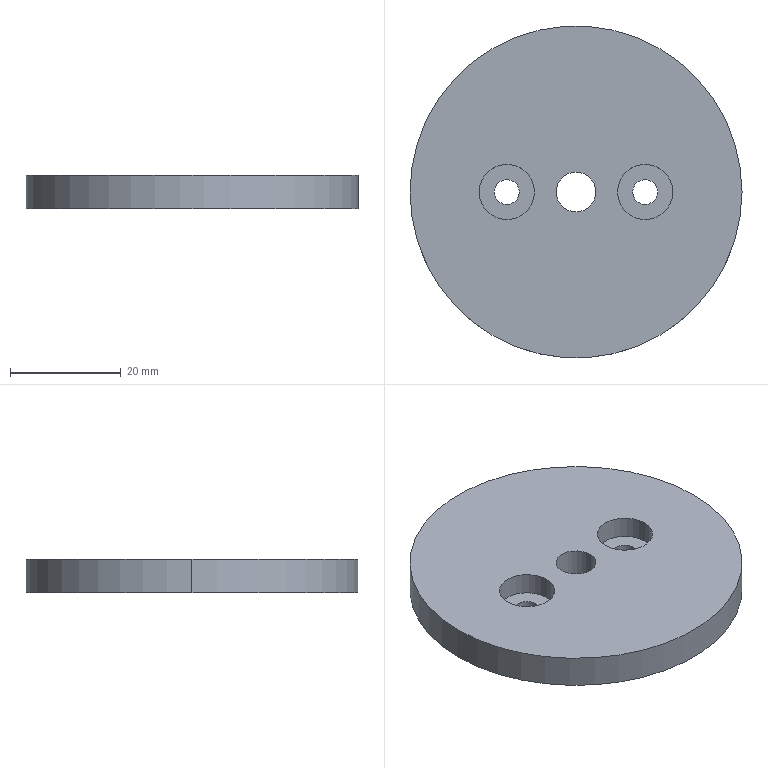Part | SolidWorks | features Extrusion 1, HoleWzd 1, ICE 1 | 1 solid | 16 faces | box 60 x 60 x 6 mm | volume 16028 mm3 | cylinder 12 | plane 4 | commonest cylinder face diameters 4.5 x4 10 x4 7.2 x2 60 x2
STEP:
#1=CARTESIAN_POINT('',(-3.6,0.,0.));
#2=VERTEX_POINT('',#1);
#3=CARTESIAN_POINT('',(3.6,0.,0.));
#4=VERTEX_POINT('',#3);
#5=CARTESIAN_POINT('',(0.,0.,0.));
#6=DIRECTION('',(0.,0.,1.));
#7=DIRECTION('',(1.,0.,0.));
#8=AXIS2_PLACEMENT_3D('',#5,#6,#7);
#9=CIRCLE('',#8,3.6);
#10=EDGE_CURVE('',#2,#4,#9,.T.);
#11=ORIENTED_EDGE('',*,*,#10,.F.);
#12=CARTESIAN_POINT('',(-3.6,0.,6.));
#13=VERTEX_POINT('',#12);
#14=CARTESIAN_POINT('',(-3.6,0.,-4.));
#15=DIRECTION('',(0.,0.,1.));
#16=VECTOR('',#15,1000.);
#17=LINE('',#14,#16);
#18=EDGE_CURVE('',#2,#13,#17,.T.);
#19=ORIENTED_EDGE('',*,*,#18,.T.);
#20=CARTESIAN_POINT('',(3.6,0.,6.));
#21=VERTEX_POINT('',#20);
#22=CARTESIAN_POINT('',(0.,0.,6.));
#23=DIRECTION('',(0.,0.,1.));
#24=DIRECTION('',(1.,0.,0.));
#25=AXIS2_PLACEMENT_3D('',#22,#23,#24);
#26=CIRCLE('',#25,3.6);
#27=EDGE_CURVE('',#13,#21,#26,.T.);
#28=ORIENTED_EDGE('',*,*,#27,.T.);
#29=CARTESIAN_POINT('',(3.6,0.,-4.));
#30=DIRECTION('',(0.,0.,1.));
#31=VECTOR('',#30,1000.);
#32=LINE('',#29,#31);
#33=EDGE_CURVE('',#4,#21,#32,.T.);
#34=ORIENTED_EDGE('',*,*,#33,.F.);
#35=EDGE_LOOP('',(#11,#19,#28,#34));
#36=FACE_OUTER_BOUND('',#35,.T.);
#37=CARTESIAN_POINT('',(0.,0.,-4.));
#38=DIRECTION('',(0.,0.,1.));
#39=DIRECTION('',(1.,0.,0.));
#40=AXIS2_PLACEMENT_3D('',#37,#38,#39);
#41=CYLINDRICAL_SURFACE('',#40,3.6);
#42=ADVANCED_FACE('',(#36),#41,.F.);
#43=CARTESIAN_POINT('',(-17.5,0.,2.));
#44=VERTEX_POINT('',#43);
#45=CARTESIAN_POINT('',(-7.5,0.,2.));
#46=VERTEX_POINT('',#45);
#47=CARTESIAN_POINT('',(-12.5,0.,2.));
#48=DIRECTION('',(0.,0.,1.));
#49=DIRECTION('',(1.,0.,0.));
#50=AXIS2_PLACEMENT_3D('',#47,#48,#49);
#51=CIRCLE('',#50,5.);
#52=EDGE_CURVE('',#44,#46,#51,.T.);
#53=ORIENTED_EDGE('',*,*,#52,.F.);
#54=CARTESIAN_POINT('',(-17.5,0.,6.));
#55=VERTEX_POINT('',#54);
#56=CARTESIAN_POINT('',(-17.5,0.,6.));
#57=DIRECTION('',(0.,0.,1.));
#58=VECTOR('',#57,1000.);
#59=LINE('',#56,#58);
#60=EDGE_CURVE('',#44,#55,#59,.T.);
#61=ORIENTED_EDGE('',*,*,#60,.T.);
#62=CARTESIAN_POINT('',(-7.5,0.,6.));
#63=VERTEX_POINT('',#62);
#64=CARTESIAN_POINT('',(-12.5,0.,6.));
#65=DIRECTION('',(0.,0.,1.));
#66=DIRECTION('',(1.,0.,0.));
#67=AXIS2_PLACEMENT_3D('',#64,#65,#66);
#68=CIRCLE('',#67,5.);
#69=EDGE_CURVE('',#55,#63,#68,.T.);
#70=ORIENTED_EDGE('',*,*,#69,.T.);
#71=CARTESIAN_POINT('',(-7.5,0.,6.));
#72=DIRECTION('',(0.,0.,1.));
#73=VECTOR('',#72,1000.);
#74=LINE('',#71,#73);
#75=EDGE_CURVE('',#46,#63,#74,.T.);
#76=ORIENTED_EDGE('',*,*,#75,.F.);
#77=EDGE_LOOP('',(#53,#61,#70,#76));
#78=FACE_OUTER_BOUND('',#77,.T.);
#79=CARTESIAN_POINT('',(-12.5,0.,6.));
#80=DIRECTION('',(0.,0.,1.));
#81=DIRECTION('',(1.,0.,0.));
#82=AXIS2_PLACEMENT_3D('',#79,#80,#81);
#83=CYLINDRICAL_SURFACE('',#82,5.);
#84=ADVANCED_FACE('',(#78),#83,.F.);
#85=CARTESIAN_POINT('',(-14.75,0.,0.));
#86=VERTEX_POINT('',#85);
#87=CARTESIAN_POINT('',(-10.25,0.,0.));
#88=VERTEX_POINT('',#87);
#89=CARTESIAN_POINT('',(-12.5,0.,0.));
#90=DIRECTION('',(0.,0.,1.));
#91=DIRECTION('',(1.,0.,0.));
#92=AXIS2_PLACEMENT_3D('',#89,#90,#91);
#93=CIRCLE('',#92,2.25);
#94=EDGE_CURVE('',#86,#88,#93,.T.);
#95=ORIENTED_EDGE('',*,*,#94,.F.);
#96=CARTESIAN_POINT('',(-14.75,0.,2.));
#97=VERTEX_POINT('',#96);
#98=CARTESIAN_POINT('',(-14.75,0.,6.));
#99=DIRECTION('',(0.,0.,1.));
#100=VECTOR('',#99,1000.);
#101=LINE('',#98,#100);
#102=EDGE_CURVE('',#86,#97,#101,.T.);
#103=ORIENTED_EDGE('',*,*,#102,.T.);
#104=CARTESIAN_POINT('',(-10.25,0.,2.));
#105=VERTEX_POINT('',#104);
#106=CARTESIAN_POINT('',(-12.5,0.,2.));
#107=DIRECTION('',(0.,0.,1.));
#108=DIRECTION('',(1.,0.,0.));
#109=AXIS2_PLACEMENT_3D('',#106,#107,#108);
#110=CIRCLE('',#109,2.25);
#111=EDGE_CURVE('',#97,#105,#110,.T.);
#112=ORIENTED_EDGE('',*,*,#111,.T.);
#113=CARTESIAN_POINT('',(-10.25,0.,6.));
#114=DIRECTION('',(0.,0.,1.));
#115=VECTOR('',#114,1000.);
#116=LINE('',#113,#115);
#117=EDGE_CURVE('',#88,#105,#116,.T.);
#118=ORIENTED_EDGE('',*,*,#117,.F.);
#119=EDGE_LOOP('',(#95,#103,#112,#118));
#120=FACE_OUTER_BOUND('',#119,.T.);
#121=CARTESIAN_POINT('',(-12.5,0.,6.));
#122=DIRECTION('',(0.,0.,1.));
#123=DIRECTION('',(1.,0.,0.));
#124=AXIS2_PLACEMENT_3D('',#121,#122,#123);
#125=CYLINDRICAL_SURFACE('',#124,2.25);
#126=ADVANCED_FACE('',(#120),#125,.F.);
#127=CARTESIAN_POINT('',(7.5,0.,2.));
#128=VERTEX_POINT('',#127);
#129=CARTESIAN_POINT('',(17.5,0.,2.));
#130=VERTEX_POINT('',#129);
#131=CARTESIAN_POINT('',(12.5,0.,2.));
#132=DIRECTION('',(0.,0.,1.));
#133=DIRECTION('',(1.,0.,0.));
#134=AXIS2_PLACEMENT_3D('',#131,#132,#133);
#135=CIRCLE('',#134,5.);
#136=EDGE_CURVE('',#128,#130,#135,.T.);
#137=ORIENTED_EDGE('',*,*,#136,.F.);
#138=CARTESIAN_POINT('',(7.5,0.,6.));
#139=VERTEX_POINT('',#138);
#140=CARTESIAN_POINT('',(7.5,0.,6.));
#141=DIRECTION('',(0.,0.,1.));
#142=VECTOR('',#141,1000.);
#143=LINE('',#140,#142);
#144=EDGE_CURVE('',#128,#139,#143,.T.);
#145=ORIENTED_EDGE('',*,*,#144,.T.);
#146=CARTESIAN_POINT('',(17.5,0.,6.));
#147=VERTEX_POINT('',#146);
#148=CARTESIAN_POINT('',(12.5,0.,6.));
#149=DIRECTION('',(0.,0.,1.));
#150=DIRECTION('',(1.,0.,0.));
#151=AXIS2_PLACEMENT_3D('',#148,#149,#150);
#152=CIRCLE('',#151,5.);
#153=EDGE_CURVE('',#139,#147,#152,.T.);
#154=ORIENTED_EDGE('',*,*,#153,.T.);
#155=CARTESIAN_POINT('',(17.5,0.,6.));
#156=DIRECTION('',(0.,0.,1.));
#157=VECTOR('',#156,1000.);
#158=LINE('',#155,#157);
#159=EDGE_CURVE('',#130,#147,#158,.T.);
#160=ORIENTED_EDGE('',*,*,#159,.F.);
#161=EDGE_LOOP('',(#137,#145,#154,#160));
#162=FACE_OUTER_BOUND('',#161,.T.);
#163=CARTESIAN_POINT('',(12.5,0.,6.));
#164=DIRECTION('',(0.,0.,1.));
#165=DIRECTION('',(1.,0.,0.));
#166=AXIS2_PLACEMENT_3D('',#163,#164,#165);
#167=CYLINDRICAL_SURFACE('',#166,5.);
#168=ADVANCED_FACE('',(#162),#167,.F.);
#169=CARTESIAN_POINT('',(10.25,0.,0.));
#170=VERTEX_POINT('',#169);
#171=CARTESIAN_POINT('',(14.75,0.,0.));
#172=VERTEX_POINT('',#171);
#173=CARTESIAN_POINT('',(12.5,0.,0.));
#174=DIRECTION('',(0.,0.,1.));
#175=DIRECTION('',(1.,0.,0.));
#176=AXIS2_PLACEMENT_3D('',#173,#174,#175);
#177=CIRCLE('',#176,2.25);
#178=EDGE_CURVE('',#170,#172,#177,.T.);
#179=ORIENTED_EDGE('',*,*,#178,.F.);
#180=CARTESIAN_POINT('',(10.25,0.,2.));
#181=VERTEX_POINT('',#180);
#182=CARTESIAN_POINT('',(10.25,0.,6.));
#183=DIRECTION('',(0.,0.,1.));
#184=VECTOR('',#183,1000.);
#185=LINE('',#182,#184);
#186=EDGE_CURVE('',#170,#181,#185,.T.);
#187=ORIENTED_EDGE('',*,*,#186,.T.);
#188=CARTESIAN_POINT('',(14.75,0.,2.));
#189=VERTEX_POINT('',#188);
#190=CARTESIAN_POINT('',(12.5,0.,2.));
#191=DIRECTION('',(0.,0.,1.));
#192=DIRECTION('',(1.,0.,0.));
#193=AXIS2_PLACEMENT_3D('',#190,#191,#192);
#194=CIRCLE('',#193,2.25);
#195=EDGE_CURVE('',#181,#189,#194,.T.);
#196=ORIENTED_EDGE('',*,*,#195,.T.);
#197=CARTESIAN_POINT('',(14.75,0.,6.));
#198=DIRECTION('',(0.,0.,1.));
#199=VECTOR('',#198,1000.);
#200=LINE('',#197,#199);
#201=EDGE_CURVE('',#172,#189,#200,.T.);
#202=ORIENTED_EDGE('',*,*,#201,.F.);
#203=EDGE_LOOP('',(#179,#187,#196,#202));
#204=FACE_OUTER_BOUND('',#203,.T.);
#205=CARTESIAN_POINT('',(12.5,0.,6.));
#206=DIRECTION('',(0.,0.,1.));
#207=DIRECTION('',(1.,0.,0.));
#208=AXIS2_PLACEMENT_3D('',#205,#206,#207);
#209=CYLINDRICAL_SURFACE('',#208,2.25);
#210=ADVANCED_FACE('',(#204),#209,.F.);
#211=CARTESIAN_POINT('',(30.,0.,6.));
#212=VERTEX_POINT('',#211);
#213=CARTESIAN_POINT('',(-30.,0.,6.));
#214=VERTEX_POINT('',#213);
#215=CARTESIAN_POINT('',(0.,0.,6.));
#216=DIRECTION('',(0.,0.,1.));
#217=DIRECTION('',(1.,0.,0.));
#218=AXIS2_PLACEMENT_3D('',#215,#216,#217);
#219=CIRCLE('',#218,30.);
#220=EDGE_CURVE('',#212,#214,#219,.T.);
#221=ORIENTED_EDGE('',*,*,#220,.F.);
#222=CARTESIAN_POINT('',(30.,0.,0.));
#223=VERTEX_POINT('',#222);
#224=CARTESIAN_POINT('',(30.,0.,6.));
#225=DIRECTION('',(0.,0.,-1.));
#226=VECTOR('',#225,1000.);
#227=LINE('',#224,#226);
#228=EDGE_CURVE('',#212,#223,#227,.T.);
#229=ORIENTED_EDGE('',*,*,#228,.T.);
#230=CARTESIAN_POINT('',(-30.,0.,0.));
#231=VERTEX_POINT('',#230);
#232=CARTESIAN_POINT('',(0.,0.,0.));
#233=DIRECTION('',(0.,0.,1.));
#234=DIRECTION('',(1.,0.,0.));
#235=AXIS2_PLACEMENT_3D('',#232,#233,#234);
#236=CIRCLE('',#235,30.);
#237=EDGE_CURVE('',#223,#231,#236,.T.);
#238=ORIENTED_EDGE('',*,*,#237,.T.);
#239=CARTESIAN_POINT('',(-30.,0.,6.));
#240=DIRECTION('',(0.,0.,-1.));
#241=VECTOR('',#240,1000.);
#242=LINE('',#239,#241);
#243=EDGE_CURVE('',#214,#231,#242,.T.);
#244=ORIENTED_EDGE('',*,*,#243,.F.);
#245=EDGE_LOOP('',(#221,#229,#238,#244));
#246=FACE_OUTER_BOUND('',#245,.T.);
#247=CARTESIAN_POINT('',(0.,0.,6.));
#248=DIRECTION('',(0.,0.,-1.));
#249=DIRECTION('',(-1.,0.,0.));
#250=AXIS2_PLACEMENT_3D('',#247,#248,#249);
#251=CYLINDRICAL_SURFACE('',#250,30.);
#252=ADVANCED_FACE('',(#246),#251,.T.);
#253=ORIENTED_EDGE('',*,*,#228,.F.);
#254=CARTESIAN_POINT('',(0.,0.,6.));
#255=DIRECTION('',(0.,0.,1.));
#256=DIRECTION('',(1.,0.,0.));
#257=AXIS2_PLACEMENT_3D('',#254,#255,#256);
#258=CIRCLE('',#257,30.);
#259=EDGE_CURVE('',#214,#212,#258,.T.);
#260=ORIENTED_EDGE('',*,*,#259,.F.);
#261=ORIENTED_EDGE('',*,*,#243,.T.);
#262=CARTESIAN_POINT('',(0.,0.,0.));
#263=DIRECTION('',(0.,0.,1.));
#264=DIRECTION('',(1.,0.,0.));
#265=AXIS2_PLACEMENT_3D('',#262,#263,#264);
#266=CIRCLE('',#265,30.);
#267=EDGE_CURVE('',#231,#223,#266,.T.);
#268=ORIENTED_EDGE('',*,*,#267,.T.);
#269=EDGE_LOOP('',(#253,#260,#261,#268));
#270=FACE_OUTER_BOUND('',#269,.T.);
#271=CARTESIAN_POINT('',(0.,0.,6.));
#272=DIRECTION('',(0.,0.,-1.));
#273=DIRECTION('',(-1.,0.,0.));
#274=AXIS2_PLACEMENT_3D('',#271,#272,#273);
#275=CYLINDRICAL_SURFACE('',#274,30.);
#276=ADVANCED_FACE('',(#270),#275,.T.);
#277=CARTESIAN_POINT('',(0.,0.,6.));
#278=DIRECTION('',(0.,0.,1.));
#279=DIRECTION('',(1.,0.,0.));
#280=AXIS2_PLACEMENT_3D('',#277,#278,#279);
#281=CIRCLE('',#280,3.6);
#282=EDGE_CURVE('',#21,#13,#281,.T.);
#283=ORIENTED_EDGE('',*,*,#282,.F.);
#284=ORIENTED_EDGE('',*,*,#27,.F.);
#285=EDGE_LOOP('',(#283,#284));
#286=FACE_BOUND('',#285,.T.);
#287=CARTESIAN_POINT('',(-12.5,0.,6.));
#288=DIRECTION('',(0.,0.,1.));
#289=DIRECTION('',(1.,0.,0.));
#290=AXIS2_PLACEMENT_3D('',#287,#288,#289);
#291=CIRCLE('',#290,5.);
#292=EDGE_CURVE('',#63,#55,#291,.T.);
#293=ORIENTED_EDGE('',*,*,#292,.F.);
#294=ORIENTED_EDGE('',*,*,#69,.F.);
#295=EDGE_LOOP('',(#293,#294));
#296=FACE_BOUND('',#295,.T.);
#297=CARTESIAN_POINT('',(12.5,0.,6.));
#298=DIRECTION('',(0.,0.,1.));
#299=DIRECTION('',(1.,0.,0.));
#300=AXIS2_PLACEMENT_3D('',#297,#298,#299);
#301=CIRCLE('',#300,5.);
#302=EDGE_CURVE('',#147,#139,#301,.T.);
#303=ORIENTED_EDGE('',*,*,#302,.F.);
#304=ORIENTED_EDGE('',*,*,#153,.F.);
#305=EDGE_LOOP('',(#303,#304));
#306=FACE_BOUND('',#305,.T.);
#307=ORIENTED_EDGE('',*,*,#259,.T.);
#308=ORIENTED_EDGE('',*,*,#220,.T.);
#309=EDGE_LOOP('',(#307,#308));
#310=FACE_OUTER_BOUND('',#309,.T.);
#311=CARTESIAN_POINT('',(0.,0.,6.));
#312=DIRECTION('',(0.,0.,1.));
#313=DIRECTION('',(1.,0.,0.));
#314=AXIS2_PLACEMENT_3D('',#311,#312,#313);
#315=PLANE('',#314);
#316=ADVANCED_FACE('',(#286,#296,#306,#310),#315,.T.);
#317=CARTESIAN_POINT('',(0.,0.,0.));
#318=DIRECTION('',(0.,0.,1.));
#319=DIRECTION('',(1.,0.,0.));
#320=AXIS2_PLACEMENT_3D('',#317,#318,#319);
#321=CIRCLE('',#320,3.6);
#322=EDGE_CURVE('',#4,#2,#321,.T.);
#323=ORIENTED_EDGE('',*,*,#322,.T.);
#324=ORIENTED_EDGE('',*,*,#10,.T.);
#325=EDGE_LOOP('',(#323,#324));
#326=FACE_BOUND('',#325,.T.);
#327=CARTESIAN_POINT('',(-12.5,0.,0.));
#328=DIRECTION('',(0.,0.,1.));
#329=DIRECTION('',(1.,0.,0.));
#330=AXIS2_PLACEMENT_3D('',#327,#328,#329);
#331=CIRCLE('',#330,2.25);
#332=EDGE_CURVE('',#88,#86,#331,.T.);
#333=ORIENTED_EDGE('',*,*,#332,.T.);
#334=ORIENTED_EDGE('',*,*,#94,.T.);
#335=EDGE_LOOP('',(#333,#334));
#336=FACE_BOUND('',#335,.T.);
#337=CARTESIAN_POINT('',(12.5,0.,0.));
#338=DIRECTION('',(0.,0.,1.));
#339=DIRECTION('',(1.,0.,0.));
#340=AXIS2_PLACEMENT_3D('',#337,#338,#339);
#341=CIRCLE('',#340,2.25);
#342=EDGE_CURVE('',#172,#170,#341,.T.);
#343=ORIENTED_EDGE('',*,*,#342,.T.);
#344=ORIENTED_EDGE('',*,*,#178,.T.);
#345=EDGE_LOOP('',(#343,#344));
#346=FACE_BOUND('',#345,.T.);
#347=ORIENTED_EDGE('',*,*,#267,.F.);
#348=ORIENTED_EDGE('',*,*,#237,.F.);
#349=EDGE_LOOP('',(#347,#348));
#350=FACE_OUTER_BOUND('',#349,.T.);
#351=CARTESIAN_POINT('',(0.,0.,0.));
#352=DIRECTION('',(0.,0.,1.));
#353=DIRECTION('',(1.,0.,0.));
#354=AXIS2_PLACEMENT_3D('',#351,#352,#353);
#355=PLANE('',#354);
#356=ADVANCED_FACE('',(#326,#336,#346,#350),#355,.F.);
#357=ORIENTED_EDGE('',*,*,#186,.F.);
#358=ORIENTED_EDGE('',*,*,#342,.F.);
#359=ORIENTED_EDGE('',*,*,#201,.T.);
#360=CARTESIAN_POINT('',(12.5,0.,2.));
#361=DIRECTION('',(0.,0.,1.));
#362=DIRECTION('',(1.,0.,0.));
#363=AXIS2_PLACEMENT_3D('',#360,#361,#362);
#364=CIRCLE('',#363,2.25);
#365=EDGE_CURVE('',#189,#181,#364,.T.);
#366=ORIENTED_EDGE('',*,*,#365,.T.);
#367=EDGE_LOOP('',(#357,#358,#359,#366));
#368=FACE_OUTER_BOUND('',#367,.T.);
#369=CARTESIAN_POINT('',(12.5,0.,6.));
#370=DIRECTION('',(0.,0.,1.));
#371=DIRECTION('',(1.,0.,0.));
#372=AXIS2_PLACEMENT_3D('',#369,#370,#371);
#373=CYLINDRICAL_SURFACE('',#372,2.25);
#374=ADVANCED_FACE('',(#368),#373,.F.);
#375=ORIENTED_EDGE('',*,*,#365,.F.);
#376=ORIENTED_EDGE('',*,*,#195,.F.);
#377=EDGE_LOOP('',(#375,#376));
#378=FACE_BOUND('',#377,.T.);
#379=CARTESIAN_POINT('',(12.5,0.,2.));
#380=DIRECTION('',(0.,0.,1.));
#381=DIRECTION('',(1.,0.,0.));
#382=AXIS2_PLACEMENT_3D('',#379,#380,#381);
#383=CIRCLE('',#382,5.);
#384=EDGE_CURVE('',#130,#128,#383,.T.);
#385=ORIENTED_EDGE('',*,*,#384,.T.);
#386=ORIENTED_EDGE('',*,*,#136,.T.);
#387=EDGE_LOOP('',(#385,#386));
#388=FACE_OUTER_BOUND('',#387,.T.);
#389=CARTESIAN_POINT('',(14.75,0.,2.));
#390=DIRECTION('',(0.,0.,-1.));
#391=DIRECTION('',(-1.,0.,0.));
#392=AXIS2_PLACEMENT_3D('',#389,#390,#391);
#393=PLANE('',#392);
#394=ADVANCED_FACE('',(#378,#388),#393,.F.);
#395=ORIENTED_EDGE('',*,*,#144,.F.);
#396=ORIENTED_EDGE('',*,*,#384,.F.);
#397=ORIENTED_EDGE('',*,*,#159,.T.);
#398=ORIENTED_EDGE('',*,*,#302,.T.);
#399=EDGE_LOOP('',(#395,#396,#397,#398));
#400=FACE_OUTER_BOUND('',#399,.T.);
#401=CARTESIAN_POINT('',(12.5,0.,6.));
#402=DIRECTION('',(0.,0.,1.));
#403=DIRECTION('',(1.,0.,0.));
#404=AXIS2_PLACEMENT_3D('',#401,#402,#403);
#405=CYLINDRICAL_SURFACE('',#404,5.);
#406=ADVANCED_FACE('',(#400),#405,.F.);
#407=ORIENTED_EDGE('',*,*,#102,.F.);
#408=ORIENTED_EDGE('',*,*,#332,.F.);
#409=ORIENTED_EDGE('',*,*,#117,.T.);
#410=CARTESIAN_POINT('',(-12.5,0.,2.));
#411=DIRECTION('',(0.,0.,1.));
#412=DIRECTION('',(1.,0.,0.));
#413=AXIS2_PLACEMENT_3D('',#410,#411,#412);
#414=CIRCLE('',#413,2.25);
#415=EDGE_CURVE('',#105,#97,#414,.T.);
#416=ORIENTED_EDGE('',*,*,#415,.T.);
#417=EDGE_LOOP('',(#407,#408,#409,#416));
#418=FACE_OUTER_BOUND('',#417,.T.);
#419=CARTESIAN_POINT('',(-12.5,0.,6.));
#420=DIRECTION('',(0.,0.,1.));
#421=DIRECTION('',(1.,0.,0.));
#422=AXIS2_PLACEMENT_3D('',#419,#420,#421);
#423=CYLINDRICAL_SURFACE('',#422,2.25);
#424=ADVANCED_FACE('',(#418),#423,.F.);
#425=ORIENTED_EDGE('',*,*,#415,.F.);
#426=ORIENTED_EDGE('',*,*,#111,.F.);
#427=EDGE_LOOP('',(#425,#426));
#428=FACE_BOUND('',#427,.T.);
#429=CARTESIAN_POINT('',(-12.5,0.,2.));
#430=DIRECTION('',(0.,0.,1.));
#431=DIRECTION('',(1.,0.,0.));
#432=AXIS2_PLACEMENT_3D('',#429,#430,#431);
#433=CIRCLE('',#432,5.);
#434=EDGE_CURVE('',#46,#44,#433,.T.);
#435=ORIENTED_EDGE('',*,*,#434,.T.);
#436=ORIENTED_EDGE('',*,*,#52,.T.);
#437=EDGE_LOOP('',(#435,#436));
#438=FACE_OUTER_BOUND('',#437,.T.);
#439=CARTESIAN_POINT('',(-10.25,0.,2.));
#440=DIRECTION('',(0.,0.,-1.));
#441=DIRECTION('',(-1.,0.,0.));
#442=AXIS2_PLACEMENT_3D('',#439,#440,#441);
#443=PLANE('',#442);
#444=ADVANCED_FACE('',(#428,#438),#443,.F.);
#445=ORIENTED_EDGE('',*,*,#60,.F.);
#446=ORIENTED_EDGE('',*,*,#434,.F.);
#447=ORIENTED_EDGE('',*,*,#75,.T.);
#448=ORIENTED_EDGE('',*,*,#292,.T.);
#449=EDGE_LOOP('',(#445,#446,#447,#448));
#450=FACE_OUTER_BOUND('',#449,.T.);
#451=CARTESIAN_POINT('',(-12.5,0.,6.));
#452=DIRECTION('',(0.,0.,1.));
#453=DIRECTION('',(1.,0.,0.));
#454=AXIS2_PLACEMENT_3D('',#451,#452,#453);
#455=CYLINDRICAL_SURFACE('',#454,5.);
#456=ADVANCED_FACE('',(#450),#455,.F.);
#457=ORIENTED_EDGE('',*,*,#18,.F.);
#458=ORIENTED_EDGE('',*,*,#322,.F.);
#459=ORIENTED_EDGE('',*,*,#33,.T.);
#460=ORIENTED_EDGE('',*,*,#282,.T.);
#461=EDGE_LOOP('',(#457,#458,#459,#460));
#462=FACE_OUTER_BOUND('',#461,.T.);
#463=CARTESIAN_POINT('',(0.,0.,-4.));
#464=DIRECTION('',(0.,0.,1.));
#465=DIRECTION('',(1.,0.,0.));
#466=AXIS2_PLACEMENT_3D('',#463,#464,#465);
#467=CYLINDRICAL_SURFACE('',#466,3.6);
#468=ADVANCED_FACE('',(#462),#467,.F.);
#469=CLOSED_SHELL('',(#42,#84,#126,#168,#210,#252,#276,#316,#356,#374,#394,#406,#424,#444,#456,#468));
#470=MANIFOLD_SOLID_BREP('',#469);
#471=CARTESIAN_POINT('',(0.,0.,0.));
#472=DIRECTION('',(0.,0.,1.));
#473=DIRECTION('',(1.,0.,0.));
#474=AXIS2_PLACEMENT_3D('',#471,#472,#473);
#475=(LENGTH_UNIT()NAMED_UNIT(*)SI_UNIT(.MILLI.,.METRE.));
#476=UNCERTAINTY_MEASURE_WITH_UNIT(LENGTH_MEASURE(0.00001),#475,'','');
#477=(NAMED_UNIT(*)PLANE_ANGLE_UNIT()SI_UNIT($,.RADIAN.));
#478=(NAMED_UNIT(*)SI_UNIT($,.STERADIAN.)SOLID_ANGLE_UNIT());
#479=(GEOMETRIC_REPRESENTATION_CONTEXT(3)GLOBAL_UNCERTAINTY_ASSIGNED_CONTEXT((#476))GLOBAL_UNIT_ASSIGNED_CONTEXT((#475,#477,#478))REPRESENTATION_CONTEXT('',''));
#480=ADVANCED_BREP_SHAPE_REPRESENTATION('',(#470,#474),#479);